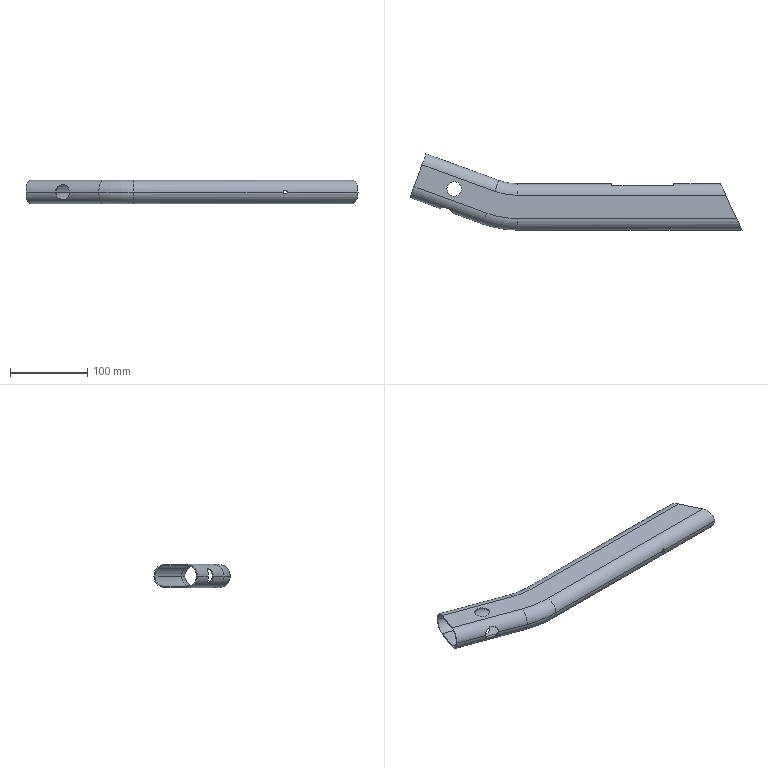Part | STEP file | 7471201 | 1 solid | 38 faces | box 428.432 x 98.424 x 30 mm | volume 88496 mm3 | cylinder 20 | plane 10 | torus 8 | commonest cylinder face diameters 27 x8 30 x8 19 x3 5 x1